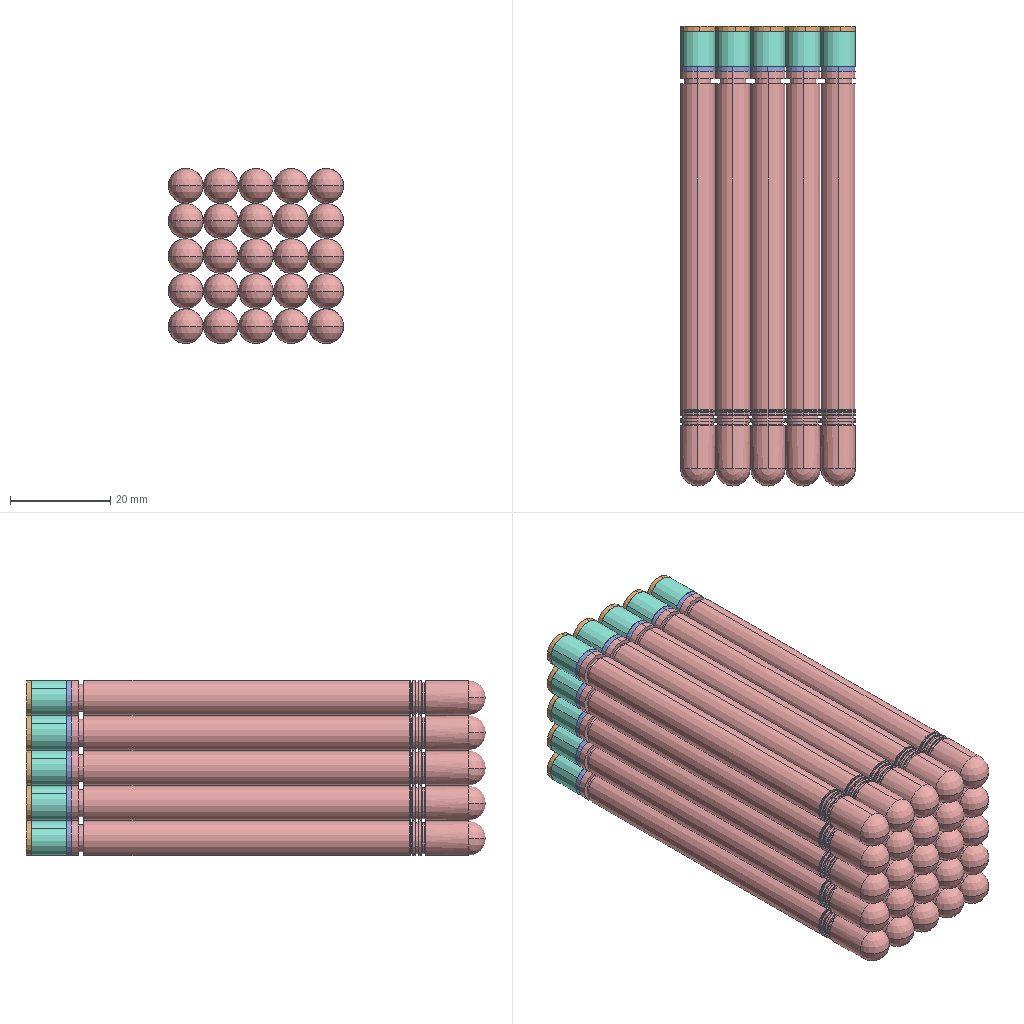Assembly | SolidWorks | 6 different items | 150 placed | box 35 x 92 x 35 mm
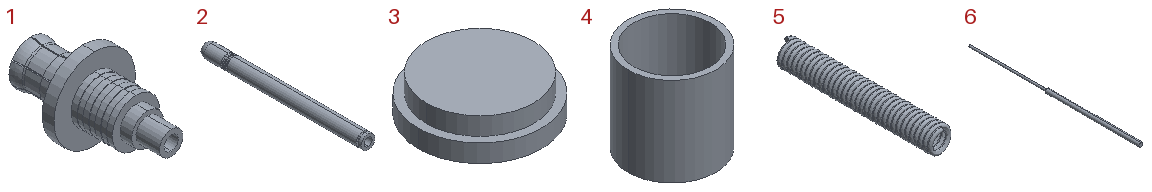Parts list (item | quantity | size | volume | features):
1 | x25 | 6.9 x 11.9 x 6.9 mm | 89.557 mm3 | features ICE 4, CirPattern 1, Revolution 1
2 | x25 | 6.9 x 82.6 x 6.9 mm | 2024 mm3 | features Revolution 1
3 | x25 | 6.9 x 6.9 x 2 mm | 65.667 mm3 | features Extrusion 1, ICE 1
4 | x25 | 6.9 x 6.9 x 7 mm | 63.829 mm3 | features Extrusion 1
5 | x25 | 3 x 19.2 x 3 mm | 52.414 mm3 | features Helix 1, Sweep 1
6 | x25 | 1.75 x 73 x 1.75 mm | 117.205 mm3 | features Extrusion 1, ICE 1
Mates (type | each side: item.copy, entity, surface, feature):
Concentric | 2.1 face cylinder Revolve1 | 1.1 face cylinder Revolve1
Coincident | 2.1 face plane Revolve1 | 1.1 face plane Revolve1
Coincident | 2.1 plane | 1.1 plane
Concentric | 1.1 face cylinder Revolve1 | 6.1 face cylinder Boss-Extrude1
Coincident | 1.1 face plane Revolve1 | 6.1 face plane Boss-Extrude1
Concentric | 6.1 face cylinder Boss-Extrude1 | 5.1 select_type:24
Coordinate | 1.1 select_type:25 | assembly select_type:11
Coincident | 6.1 face plane Boss-Extrude1 | 5.1 select_type:24
Concentric | 1.1 face cylinder Revolve1 | 4.1 face cylinder Boss-Extrude1
Coincident | 1.1 face plane Revolve1 | 4.1 face plane Boss-Extrude1
Concentric | 4.1 face cylinder Boss-Extrude1 | 3.1 face cylinder Boss-Extrude1
Coincident | 4.1 face plane Boss-Extrude1 | 3.1 face plane Boss-Extrude2